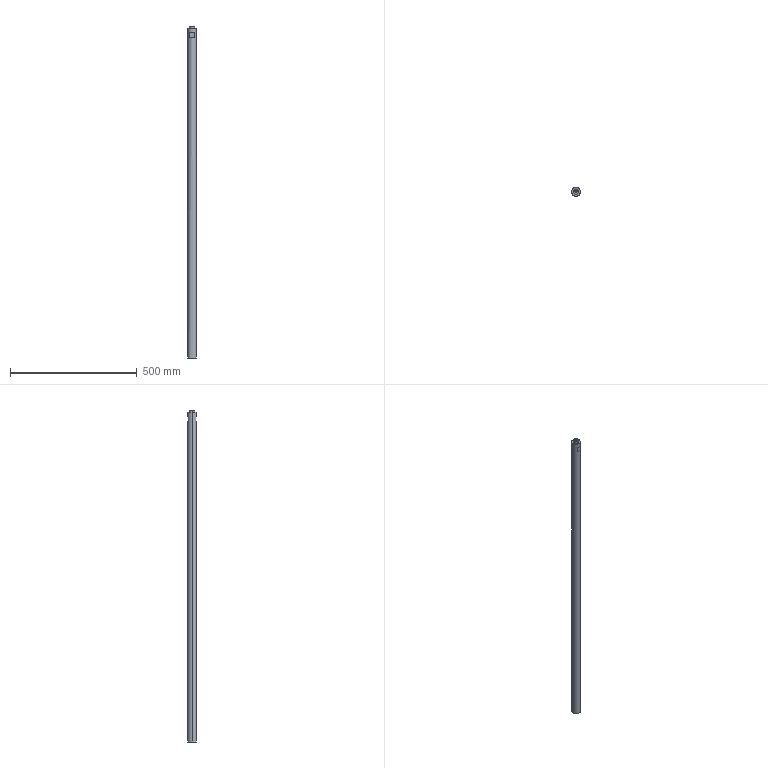Part | STEP file | 44-02-05 Press-fit Guide Shaft | 1 solid | 21 faces | box 35 x 35 x 1310 mm | volume 1250098 mm3 | plane 9 | cylinder 8 | cone 4 | commonest cylinder face diameters 8.5 x4 20 x2 35 x2
STEP:
#1=CARTESIAN_POINT('',(0.,0.,0.));
#2=DIRECTION('',(0.,0.,1.));
#3=DIRECTION('',(1.,0.,0.));
#4=AXIS2_PLACEMENT_3D('',#1,#2,#3);
#5=CARTESIAN_POINT('',(4.25,0.,627.5));
#6=VERTEX_POINT('',#5);
#7=CARTESIAN_POINT('',(4.25,0.,655.));
#8=VERTEX_POINT('',#7);
#9=CARTESIAN_POINT('',(4.25,0.,655.));
#10=DIRECTION('',(0.,0.,1.));
#11=VECTOR('',#10,1.);
#12=LINE('',#9,#11);
#13=CARTESIAN_POINT('',(0.,0.,655.));
#14=DIRECTION('',(0.,0.,1.));
#15=DIRECTION('',(1.,0.,0.));
#16=AXIS2_PLACEMENT_3D('',#13,#14,#15);
#17=CYLINDRICAL_SURFACE('',#16,4.25);
#18=CARTESIAN_POINT('',(6.283,0.));
#19=DIRECTION('',(0.,1.));
#20=VECTOR('',#19,1.);
#21=LINE('',#18,#20);
#22=(GEOMETRIC_REPRESENTATION_CONTEXT(2)PARAMETRIC_REPRESENTATION_CONTEXT()REPRESENTATION_CONTEXT('',''));
#23=DEFINITIONAL_REPRESENTATION('',(#21),#22);
#24=PCURVE('',#17,#23);
#25=CARTESIAN_POINT('',(0.,0.,655.));
#26=DIRECTION('',(0.,0.,1.));
#27=DIRECTION('',(1.,0.,0.));
#28=AXIS2_PLACEMENT_3D('',#25,#26,#27);
#29=CYLINDRICAL_SURFACE('',#28,4.25);
#30=CARTESIAN_POINT('',(0.,0.));
#31=DIRECTION('',(0.,1.));
#32=VECTOR('',#31,1.);
#33=LINE('',#30,#32);
#34=(GEOMETRIC_REPRESENTATION_CONTEXT(2)PARAMETRIC_REPRESENTATION_CONTEXT()REPRESENTATION_CONTEXT('',''));
#35=DEFINITIONAL_REPRESENTATION('',(#33),#34);
#36=PCURVE('',#29,#35);
#37=SURFACE_CURVE('',#12,(#24,#36),.PCURVE_S1.);
#38=EDGE_CURVE('',#6,#8,#37,.T.);
#39=ORIENTED_EDGE('',*,*,#38,.T.);
#40=CARTESIAN_POINT('',(-4.25,0.,655.));
#41=VERTEX_POINT('',#40);
#42=CARTESIAN_POINT('',(0.,0.,655.));
#43=DIRECTION('',(0.,0.,1.));
#44=DIRECTION('',(1.,0.,0.));
#45=AXIS2_PLACEMENT_3D('',#42,#43,#44);
#46=CIRCLE('',#45,4.25);
#47=CARTESIAN_POINT('',(0.,0.));
#48=DIRECTION('',(1.,0.));
#49=VECTOR('',#48,1.);
#50=LINE('',#47,#49);
#51=(GEOMETRIC_REPRESENTATION_CONTEXT(2)PARAMETRIC_REPRESENTATION_CONTEXT()REPRESENTATION_CONTEXT('',''));
#52=DEFINITIONAL_REPRESENTATION('',(#50),#51);
#53=PCURVE('',#17,#52);
#54=CARTESIAN_POINT('',(0.,0.,655.));
#55=DIRECTION('',(0.,0.,1.));
#56=DIRECTION('',(1.,0.,0.));
#57=AXIS2_PLACEMENT_3D('',#54,#55,#56);
#58=PLANE('',#57);
#59=CARTESIAN_POINT('',(0.,0.));
#60=DIRECTION('',(1.,0.));
#61=AXIS2_PLACEMENT_2D('',#59,#60);
#62=CIRCLE('',#61,4.25);
#63=(GEOMETRIC_REPRESENTATION_CONTEXT(2)PARAMETRIC_REPRESENTATION_CONTEXT()REPRESENTATION_CONTEXT('',''));
#64=DEFINITIONAL_REPRESENTATION('',(#62),#63);
#65=PCURVE('',#58,#64);
#66=SURFACE_CURVE('',#46,(#53,#65),.PCURVE_S1.);
#67=EDGE_CURVE('',#41,#8,#66,.T.);
#68=ORIENTED_EDGE('',*,*,#67,.F.);
#69=CARTESIAN_POINT('',(-4.25,0.,627.5));
#70=VERTEX_POINT('',#69);
#71=CARTESIAN_POINT('',(-4.25,0.,655.));
#72=DIRECTION('',(0.,0.,1.));
#73=VECTOR('',#72,1.);
#74=LINE('',#71,#73);
#75=CARTESIAN_POINT('',(3.142,0.));
#76=DIRECTION('',(0.,1.));
#77=VECTOR('',#76,1.);
#78=LINE('',#75,#77);
#79=(GEOMETRIC_REPRESENTATION_CONTEXT(2)PARAMETRIC_REPRESENTATION_CONTEXT()REPRESENTATION_CONTEXT('',''));
#80=DEFINITIONAL_REPRESENTATION('',(#78),#79);
#81=PCURVE('',#17,#80);
#82=CARTESIAN_POINT('',(3.142,0.));
#83=DIRECTION('',(0.,1.));
#84=VECTOR('',#83,1.);
#85=LINE('',#82,#84);
#86=(GEOMETRIC_REPRESENTATION_CONTEXT(2)PARAMETRIC_REPRESENTATION_CONTEXT()REPRESENTATION_CONTEXT('',''));
#87=DEFINITIONAL_REPRESENTATION('',(#85),#86);
#88=PCURVE('',#29,#87);
#89=SURFACE_CURVE('',#74,(#81,#88),.PCURVE_S1.);
#90=EDGE_CURVE('',#70,#41,#89,.T.);
#91=ORIENTED_EDGE('',*,*,#90,.F.);
#92=CARTESIAN_POINT('',(0.,0.,627.5));
#93=DIRECTION('',(0.,0.,1.));
#94=DIRECTION('',(1.,0.,0.));
#95=AXIS2_PLACEMENT_3D('',#92,#93,#94);
#96=CIRCLE('',#95,4.25);
#97=CARTESIAN_POINT('',(0.,-27.5));
#98=DIRECTION('',(1.,0.));
#99=VECTOR('',#98,1.);
#100=LINE('',#97,#99);
#101=(GEOMETRIC_REPRESENTATION_CONTEXT(2)PARAMETRIC_REPRESENTATION_CONTEXT()REPRESENTATION_CONTEXT('',''));
#102=DEFINITIONAL_REPRESENTATION('',(#100),#101);
#103=PCURVE('',#17,#102);
#104=CARTESIAN_POINT('',(0.,0.,627.5));
#105=DIRECTION('',(0.,0.,1.));
#106=DIRECTION('',(1.,0.,0.));
#107=AXIS2_PLACEMENT_3D('',#104,#105,#106);
#108=CONICAL_SURFACE('',#107,4.25,1.03);
#109=CARTESIAN_POINT('',(0.,0.));
#110=DIRECTION('',(1.,0.));
#111=VECTOR('',#110,1.);
#112=LINE('',#109,#111);
#113=(GEOMETRIC_REPRESENTATION_CONTEXT(2)PARAMETRIC_REPRESENTATION_CONTEXT()REPRESENTATION_CONTEXT('',''));
#114=DEFINITIONAL_REPRESENTATION('',(#112),#113);
#115=PCURVE('',#108,#114);
#116=SURFACE_CURVE('',#96,(#103,#115),.PCURVE_S1.);
#117=EDGE_CURVE('',#70,#6,#116,.T.);
#118=ORIENTED_EDGE('',*,*,#117,.T.);
#119=EDGE_LOOP('',(#39,#68,#91,#118));
#120=FACE_BOUND('',#119,.F.);
#121=ADVANCED_FACE('',(#120),#17,.F.);
#122=ORIENTED_EDGE('',*,*,#117,.F.);
#123=CARTESIAN_POINT('',(0.,0.,624.946));
#124=VERTEX_POINT('',#123);
#125=CARTESIAN_POINT('',(-4.25,0.,627.5));
#126=DIRECTION('',(-0.8572,0.,0.515));
#127=VECTOR('',#126,1.);
#128=LINE('',#125,#127);
#129=CARTESIAN_POINT('',(3.142,0.));
#130=DIRECTION('',(0.,1.));
#131=VECTOR('',#130,1.);
#132=LINE('',#129,#131);
#133=(GEOMETRIC_REPRESENTATION_CONTEXT(2)PARAMETRIC_REPRESENTATION_CONTEXT()REPRESENTATION_CONTEXT('',''));
#134=DEFINITIONAL_REPRESENTATION('',(#132),#133);
#135=PCURVE('',#108,#134);
#136=CARTESIAN_POINT('',(0.,0.,627.5));
#137=DIRECTION('',(0.,0.,1.));
#138=DIRECTION('',(1.,0.,0.));
#139=AXIS2_PLACEMENT_3D('',#136,#137,#138);
#140=CONICAL_SURFACE('',#139,4.25,1.03);
#141=CARTESIAN_POINT('',(3.142,0.));
#142=DIRECTION('',(0.,1.));
#143=VECTOR('',#142,1.);
#144=LINE('',#141,#143);
#145=(GEOMETRIC_REPRESENTATION_CONTEXT(2)PARAMETRIC_REPRESENTATION_CONTEXT()REPRESENTATION_CONTEXT('',''));
#146=DEFINITIONAL_REPRESENTATION('',(#144),#145);
#147=PCURVE('',#140,#146);
#148=SURFACE_CURVE('',#128,(#135,#147),.PCURVE_S1.);
#149=EDGE_CURVE('',#124,#70,#148,.T.);
#150=ORIENTED_EDGE('',*,*,#149,.F.);
#151=CARTESIAN_POINT('',(4.25,0.,627.5));
#152=DIRECTION('',(0.8572,0.,0.515));
#153=VECTOR('',#152,1.);
#154=LINE('',#151,#153);
#155=CARTESIAN_POINT('',(6.283,0.));
#156=DIRECTION('',(0.,1.));
#157=VECTOR('',#156,1.);
#158=LINE('',#155,#157);
#159=(GEOMETRIC_REPRESENTATION_CONTEXT(2)PARAMETRIC_REPRESENTATION_CONTEXT()REPRESENTATION_CONTEXT('',''));
#160=DEFINITIONAL_REPRESENTATION('',(#158),#159);
#161=PCURVE('',#108,#160);
#162=CARTESIAN_POINT('',(0.,0.));
#163=DIRECTION('',(0.,1.));
#164=VECTOR('',#163,1.);
#165=LINE('',#162,#164);
#166=(GEOMETRIC_REPRESENTATION_CONTEXT(2)PARAMETRIC_REPRESENTATION_CONTEXT()REPRESENTATION_CONTEXT('',''));
#167=DEFINITIONAL_REPRESENTATION('',(#165),#166);
#168=PCURVE('',#140,#167);
#169=SURFACE_CURVE('',#154,(#161,#168),.PCURVE_S1.);
#170=EDGE_CURVE('',#124,#6,#169,.T.);
#171=ORIENTED_EDGE('',*,*,#170,.T.);
#172=EDGE_LOOP('',(#122,#150,#171));
#173=FACE_BOUND('',#172,.F.);
#174=ADVANCED_FACE('',(#173),#108,.F.);
#175=CARTESIAN_POINT('',(10.,0.,646.));
#176=VERTEX_POINT('',#175);
#177=CARTESIAN_POINT('',(-10.,0.,646.));
#178=VERTEX_POINT('',#177);
#179=CARTESIAN_POINT('',(0.,0.,646.));
#180=DIRECTION('',(0.,0.,1.));
#181=DIRECTION('',(1.,0.,0.));
#182=AXIS2_PLACEMENT_3D('',#179,#180,#181);
#183=CIRCLE('',#182,10.);
#184=CARTESIAN_POINT('',(0.,0.,646.));
#185=DIRECTION('',(0.,0.,1.));
#186=DIRECTION('',(1.,0.,0.));
#187=AXIS2_PLACEMENT_3D('',#184,#185,#186);
#188=CYLINDRICAL_SURFACE('',#187,10.);
#189=CARTESIAN_POINT('',(0.,0.));
#190=DIRECTION('',(1.,0.));
#191=VECTOR('',#190,1.);
#192=LINE('',#189,#191);
#193=(GEOMETRIC_REPRESENTATION_CONTEXT(2)PARAMETRIC_REPRESENTATION_CONTEXT()REPRESENTATION_CONTEXT('',''));
#194=DEFINITIONAL_REPRESENTATION('',(#192),#193);
#195=PCURVE('',#188,#194);
#196=CARTESIAN_POINT('',(0.,0.,646.));
#197=DIRECTION('',(0.,0.,1.));
#198=DIRECTION('',(1.,0.,0.));
#199=AXIS2_PLACEMENT_3D('',#196,#197,#198);
#200=PLANE('',#199);
#201=CARTESIAN_POINT('',(0.,0.));
#202=DIRECTION('',(1.,0.));
#203=AXIS2_PLACEMENT_2D('',#201,#202);
#204=CIRCLE('',#203,10.);
#205=(GEOMETRIC_REPRESENTATION_CONTEXT(2)PARAMETRIC_REPRESENTATION_CONTEXT()REPRESENTATION_CONTEXT('',''));
#206=DEFINITIONAL_REPRESENTATION('',(#204),#205);
#207=PCURVE('',#200,#206);
#208=SURFACE_CURVE('',#183,(#195,#207),.PCURVE_S1.);
#209=EDGE_CURVE('',#176,#178,#208,.T.);
#210=ORIENTED_EDGE('',*,*,#209,.T.);
#211=CARTESIAN_POINT('',(-10.,0.,655.));
#212=VERTEX_POINT('',#211);
#213=CARTESIAN_POINT('',(-10.,0.,646.));
#214=DIRECTION('',(0.,0.,1.));
#215=VECTOR('',#214,1.);
#216=LINE('',#213,#215);
#217=CARTESIAN_POINT('',(3.142,0.));
#218=DIRECTION('',(0.,1.));
#219=VECTOR('',#218,1.);
#220=LINE('',#217,#219);
#221=(GEOMETRIC_REPRESENTATION_CONTEXT(2)PARAMETRIC_REPRESENTATION_CONTEXT()REPRESENTATION_CONTEXT('',''));
#222=DEFINITIONAL_REPRESENTATION('',(#220),#221);
#223=PCURVE('',#188,#222);
#224=CARTESIAN_POINT('',(0.,0.,646.));
#225=DIRECTION('',(0.,0.,1.));
#226=DIRECTION('',(1.,0.,0.));
#227=AXIS2_PLACEMENT_3D('',#224,#225,#226);
#228=CYLINDRICAL_SURFACE('',#227,10.);
#229=CARTESIAN_POINT('',(3.142,0.));
#230=DIRECTION('',(0.,1.));
#231=VECTOR('',#230,1.);
#232=LINE('',#229,#231);
#233=(GEOMETRIC_REPRESENTATION_CONTEXT(2)PARAMETRIC_REPRESENTATION_CONTEXT()REPRESENTATION_CONTEXT('',''));
#234=DEFINITIONAL_REPRESENTATION('',(#232),#233);
#235=PCURVE('',#228,#234);
#236=SURFACE_CURVE('',#216,(#223,#235),.PCURVE_S1.);
#237=EDGE_CURVE('',#178,#212,#236,.T.);
#238=ORIENTED_EDGE('',*,*,#237,.T.);
#239=CARTESIAN_POINT('',(10.,0.,655.));
#240=VERTEX_POINT('',#239);
#241=CARTESIAN_POINT('',(0.,0.,655.));
#242=DIRECTION('',(0.,0.,1.));
#243=DIRECTION('',(1.,0.,0.));
#244=AXIS2_PLACEMENT_3D('',#241,#242,#243);
#245=CIRCLE('',#244,10.);
#246=CARTESIAN_POINT('',(0.,9.));
#247=DIRECTION('',(1.,0.));
#248=VECTOR('',#247,1.);
#249=LINE('',#246,#248);
#250=(GEOMETRIC_REPRESENTATION_CONTEXT(2)PARAMETRIC_REPRESENTATION_CONTEXT()REPRESENTATION_CONTEXT('',''));
#251=DEFINITIONAL_REPRESENTATION('',(#249),#250);
#252=PCURVE('',#188,#251);
#253=CARTESIAN_POINT('',(0.,0.));
#254=DIRECTION('',(1.,0.));
#255=AXIS2_PLACEMENT_2D('',#253,#254);
#256=CIRCLE('',#255,10.);
#257=(GEOMETRIC_REPRESENTATION_CONTEXT(2)PARAMETRIC_REPRESENTATION_CONTEXT()REPRESENTATION_CONTEXT('',''));
#258=DEFINITIONAL_REPRESENTATION('',(#256),#257);
#259=PCURVE('',#58,#258);
#260=SURFACE_CURVE('',#245,(#252,#259),.PCURVE_S1.);
#261=EDGE_CURVE('',#240,#212,#260,.T.);
#262=ORIENTED_EDGE('',*,*,#261,.F.);
#263=CARTESIAN_POINT('',(10.,0.,646.));
#264=DIRECTION('',(0.,0.,1.));
#265=VECTOR('',#264,1.);
#266=LINE('',#263,#265);
#267=CARTESIAN_POINT('',(0.,0.));
#268=DIRECTION('',(0.,1.));
#269=VECTOR('',#268,1.);
#270=LINE('',#267,#269);
#271=(GEOMETRIC_REPRESENTATION_CONTEXT(2)PARAMETRIC_REPRESENTATION_CONTEXT()REPRESENTATION_CONTEXT('',''));
#272=DEFINITIONAL_REPRESENTATION('',(#270),#271);
#273=PCURVE('',#188,#272);
#274=CARTESIAN_POINT('',(6.283,0.));
#275=DIRECTION('',(0.,1.));
#276=VECTOR('',#275,1.);
#277=LINE('',#274,#276);
#278=(GEOMETRIC_REPRESENTATION_CONTEXT(2)PARAMETRIC_REPRESENTATION_CONTEXT()REPRESENTATION_CONTEXT('',''));
#279=DEFINITIONAL_REPRESENTATION('',(#277),#278);
#280=PCURVE('',#228,#279);
#281=SURFACE_CURVE('',#266,(#273,#280),.PCURVE_S1.);
#282=EDGE_CURVE('',#176,#240,#281,.T.);
#283=ORIENTED_EDGE('',*,*,#282,.F.);
#284=EDGE_LOOP('',(#210,#238,#262,#283));
#285=FACE_BOUND('',#284,.T.);
#286=ADVANCED_FACE('',(#285),#188,.T.);
#287=CARTESIAN_POINT('',(-4.25,0.,-627.5));
#288=VERTEX_POINT('',#287);
#289=CARTESIAN_POINT('',(-4.25,0.,-655.));
#290=VERTEX_POINT('',#289);
#291=CARTESIAN_POINT('',(-4.25,0.,-655.));
#292=DIRECTION('',(0.,0.,-1.));
#293=VECTOR('',#292,1.);
#294=LINE('',#291,#293);
#295=CARTESIAN_POINT('',(0.,0.,-655.));
#296=DIRECTION('',(0.,0.,-1.));
#297=DIRECTION('',(-1.,0.,0.));
#298=AXIS2_PLACEMENT_3D('',#295,#296,#297);
#299=CYLINDRICAL_SURFACE('',#298,4.25);
#300=CARTESIAN_POINT('',(6.283,0.));
#301=DIRECTION('',(0.,1.));
#302=VECTOR('',#301,1.);
#303=LINE('',#300,#302);
#304=(GEOMETRIC_REPRESENTATION_CONTEXT(2)PARAMETRIC_REPRESENTATION_CONTEXT()REPRESENTATION_CONTEXT('',''));
#305=DEFINITIONAL_REPRESENTATION('',(#303),#304);
#306=PCURVE('',#299,#305);
#307=CARTESIAN_POINT('',(0.,0.,-655.));
#308=DIRECTION('',(0.,0.,-1.));
#309=DIRECTION('',(-1.,0.,0.));
#310=AXIS2_PLACEMENT_3D('',#307,#308,#309);
#311=CYLINDRICAL_SURFACE('',#310,4.25);
#312=CARTESIAN_POINT('',(0.,0.));
#313=DIRECTION('',(0.,1.));
#314=VECTOR('',#313,1.);
#315=LINE('',#312,#314);
#316=(GEOMETRIC_REPRESENTATION_CONTEXT(2)PARAMETRIC_REPRESENTATION_CONTEXT()REPRESENTATION_CONTEXT('',''));
#317=DEFINITIONAL_REPRESENTATION('',(#315),#316);
#318=PCURVE('',#311,#317);
#319=SURFACE_CURVE('',#294,(#306,#318),.PCURVE_S1.);
#320=EDGE_CURVE('',#288,#290,#319,.T.);
#321=ORIENTED_EDGE('',*,*,#320,.T.);
#322=CARTESIAN_POINT('',(4.25,0.,-655.));
#323=VERTEX_POINT('',#322);
#324=CARTESIAN_POINT('',(0.,0.,-655.));
#325=DIRECTION('',(0.,0.,-1.));
#326=DIRECTION('',(-1.,0.,0.));
#327=AXIS2_PLACEMENT_3D('',#324,#325,#326);
#328=CIRCLE('',#327,4.25);
#329=CARTESIAN_POINT('',(0.,0.));
#330=DIRECTION('',(1.,0.));
#331=VECTOR('',#330,1.);
#332=LINE('',#329,#331);
#333=(GEOMETRIC_REPRESENTATION_CONTEXT(2)PARAMETRIC_REPRESENTATION_CONTEXT()REPRESENTATION_CONTEXT('',''));
#334=DEFINITIONAL_REPRESENTATION('',(#332),#333);
#335=PCURVE('',#299,#334);
#336=CARTESIAN_POINT('',(0.,0.,-655.));
#337=DIRECTION('',(0.,0.,1.));
#338=DIRECTION('',(1.,0.,0.));
#339=AXIS2_PLACEMENT_3D('',#336,#337,#338);
#340=PLANE('',#339);
#341=CARTESIAN_POINT('',(-4.25,0.));
#342=CARTESIAN_POINT('',(-4.25,7.361));
#343=CARTESIAN_POINT('',(2.125,3.681));
#344=CARTESIAN_POINT('',(8.5,0.));
#345=CARTESIAN_POINT('',(2.125,-3.681));
#346=CARTESIAN_POINT('',(-4.25,-7.361));
#347=CARTESIAN_POINT('',(-4.25,0.));
#348=(BOUNDED_CURVE()B_SPLINE_CURVE(2,(#341,#342,#343,#344,#345,#346,#347),.UNSPECIFIED.,.T.,.F.)B_SPLINE_CURVE_WITH_KNOTS((1,2,2,2,2,1),(-2.094,0.,2.094,4.189,6.283,8.378),.UNSPECIFIED.)CURVE()GEOMETRIC_REPRESENTATION_ITEM()RATIONAL_B_SPLINE_CURVE((1.,0.5,1.,0.5,1.,0.5,1.))REPRESENTATION_ITEM(''));
#349=(GEOMETRIC_REPRESENTATION_CONTEXT(2)PARAMETRIC_REPRESENTATION_CONTEXT()REPRESENTATION_CONTEXT('',''));
#350=DEFINITIONAL_REPRESENTATION('',(#348),#349);
#351=PCURVE('',#340,#350);
#352=SURFACE_CURVE('',#328,(#335,#351),.PCURVE_S1.);
#353=EDGE_CURVE('',#323,#290,#352,.T.);
#354=ORIENTED_EDGE('',*,*,#353,.F.);
#355=CARTESIAN_POINT('',(4.25,0.,-627.5));
#356=VERTEX_POINT('',#355);
#357=CARTESIAN_POINT('',(4.25,0.,-655.));
#358=DIRECTION('',(0.,0.,-1.));
#359=VECTOR('',#358,1.);
#360=LINE('',#357,#359);
#361=CARTESIAN_POINT('',(3.142,0.));
#362=DIRECTION('',(0.,1.));
#363=VECTOR('',#362,1.);
#364=LINE('',#361,#363);
#365=(GEOMETRIC_REPRESENTATION_CONTEXT(2)PARAMETRIC_REPRESENTATION_CONTEXT()REPRESENTATION_CONTEXT('',''));
#366=DEFINITIONAL_REPRESENTATION('',(#364),#365);
#367=PCURVE('',#299,#366);
#368=CARTESIAN_POINT('',(3.142,0.));
#369=DIRECTION('',(0.,1.));
#370=VECTOR('',#369,1.);
#371=LINE('',#368,#370);
#372=(GEOMETRIC_REPRESENTATION_CONTEXT(2)PARAMETRIC_REPRESENTATION_CONTEXT()REPRESENTATION_CONTEXT('',''));
#373=DEFINITIONAL_REPRESENTATION('',(#371),#372);
#374=PCURVE('',#311,#373);
#375=SURFACE_CURVE('',#360,(#367,#374),.PCURVE_S1.);
#376=EDGE_CURVE('',#356,#323,#375,.T.);
#377=ORIENTED_EDGE('',*,*,#376,.F.);
#378=CARTESIAN_POINT('',(0.,0.,-627.5));
#379=DIRECTION('',(0.,0.,-1.));
#380=DIRECTION('',(-1.,0.,0.));
#381=AXIS2_PLACEMENT_3D('',#378,#379,#380);
#382=CIRCLE('',#381,4.25);
#383=CARTESIAN_POINT('',(0.,-27.5));
#384=DIRECTION('',(1.,0.));
#385=VECTOR('',#384,1.);
#386=LINE('',#383,#385);
#387=(GEOMETRIC_REPRESENTATION_CONTEXT(2)PARAMETRIC_REPRESENTATION_CONTEXT()REPRESENTATION_CONTEXT('',''));
#388=DEFINITIONAL_REPRESENTATION('',(#386),#387);
#389=PCURVE('',#299,#388);
#390=CARTESIAN_POINT('',(0.,0.,-627.5));
#391=DIRECTION('',(0.,0.,-1.));
#392=DIRECTION('',(-1.,0.,0.));
#393=AXIS2_PLACEMENT_3D('',#390,#391,#392);
#394=CONICAL_SURFACE('',#393,4.25,1.03);
#395=CARTESIAN_POINT('',(0.,0.));
#396=DIRECTION('',(1.,0.));
#397=VECTOR('',#396,1.);
#398=LINE('',#395,#397);
#399=(GEOMETRIC_REPRESENTATION_CONTEXT(2)PARAMETRIC_REPRESENTATION_CONTEXT()REPRESENTATION_CONTEXT('',''));
#400=DEFINITIONAL_REPRESENTATION('',(#398),#399);
#401=PCURVE('',#394,#400);
#402=SURFACE_CURVE('',#382,(#389,#401),.PCURVE_S1.);
#403=EDGE_CURVE('',#356,#288,#402,.T.);
#404=ORIENTED_EDGE('',*,*,#403,.T.);
#405=EDGE_LOOP('',(#321,#354,#377,#404));
#406=FACE_BOUND('',#405,.F.);
#407=ADVANCED_FACE('',(#406),#299,.F.);
#408=ORIENTED_EDGE('',*,*,#403,.F.);
#409=CARTESIAN_POINT('',(0.,0.,-624.946));
#410=VERTEX_POINT('',#409);
#411=CARTESIAN_POINT('',(4.25,0.,-627.5));
#412=DIRECTION('',(0.8572,0.,-0.515));
#413=VECTOR('',#412,1.);
#414=LINE('',#411,#413);
#415=CARTESIAN_POINT('',(3.142,0.));
#416=DIRECTION('',(0.,1.));
#417=VECTOR('',#416,1.);
#418=LINE('',#415,#417);
#419=(GEOMETRIC_REPRESENTATION_CONTEXT(2)PARAMETRIC_REPRESENTATION_CONTEXT()REPRESENTATION_CONTEXT('',''));
#420=DEFINITIONAL_REPRESENTATION('',(#418),#419);
#421=PCURVE('',#394,#420);
#422=CARTESIAN_POINT('',(0.,0.,-627.5));
#423=DIRECTION('',(0.,0.,-1.));
#424=DIRECTION('',(-1.,0.,0.));
#425=AXIS2_PLACEMENT_3D('',#422,#423,#424);
#426=CONICAL_SURFACE('',#425,4.25,1.03);
#427=CARTESIAN_POINT('',(3.142,0.));
#428=DIRECTION('',(0.,1.));
#429=VECTOR('',#428,1.);
#430=LINE('',#427,#429);
#431=(GEOMETRIC_REPRESENTATION_CONTEXT(2)PARAMETRIC_REPRESENTATION_CONTEXT()REPRESENTATION_CONTEXT('',''));
#432=DEFINITIONAL_REPRESENTATION('',(#430),#431);
#433=PCURVE('',#426,#432);
#434=SURFACE_CURVE('',#414,(#421,#433),.PCURVE_S1.);
#435=EDGE_CURVE('',#410,#356,#434,.T.);
#436=ORIENTED_EDGE('',*,*,#435,.F.);
#437=CARTESIAN_POINT('',(-4.25,0.,-627.5));
#438=DIRECTION('',(-0.8572,0.,-0.515));
#439=VECTOR('',#438,1.);
#440=LINE('',#437,#439);
#441=CARTESIAN_POINT('',(6.283,0.));
#442=DIRECTION('',(0.,1.));
#443=VECTOR('',#442,1.);
#444=LINE('',#441,#443);
#445=(GEOMETRIC_REPRESENTATION_CONTEXT(2)PARAMETRIC_REPRESENTATION_CONTEXT()REPRESENTATION_CONTEXT('',''));
#446=DEFINITIONAL_REPRESENTATION('',(#444),#445);
#447=PCURVE('',#394,#446);
#448=CARTESIAN_POINT('',(0.,0.));
#449=DIRECTION('',(0.,1.));
#450=VECTOR('',#449,1.);
#451=LINE('',#448,#450);
#452=(GEOMETRIC_REPRESENTATION_CONTEXT(2)PARAMETRIC_REPRESENTATION_CONTEXT()REPRESENTATION_CONTEXT('',''));
#453=DEFINITIONAL_REPRESENTATION('',(#451),#452);
#454=PCURVE('',#426,#453);
#455=SURFACE_CURVE('',#440,(#447,#454),.PCURVE_S1.);
#456=EDGE_CURVE('',#410,#288,#455,.T.);
#457=ORIENTED_EDGE('',*,*,#456,.T.);
#458=EDGE_LOOP('',(#408,#436,#457));
#459=FACE_BOUND('',#458,.F.);
#460=ADVANCED_FACE('',(#459),#394,.F.);
#461=CARTESIAN_POINT('',(9.014,15.,630.));
#462=VERTEX_POINT('',#461);
#463=CARTESIAN_POINT('',(9.014,15.,610.));
#464=VERTEX_POINT('',#463);
#465=CARTESIAN_POINT('',(9.014,15.,655.));
#466=DIRECTION('',(0.,0.,-1.));
#467=VECTOR('',#466,1.);
#468=LINE('',#465,#467);
#469=CARTESIAN_POINT('',(0.,0.,655.));
#470=DIRECTION('',(0.,0.,-1.));
#471=DIRECTION('',(-1.,0.,0.));
#472=AXIS2_PLACEMENT_3D('',#469,#470,#471);
#473=CYLINDRICAL_SURFACE('',#472,17.5);
#474=CARTESIAN_POINT('',(2.112,0.));
#475=DIRECTION('',(0.,1.));
#476=VECTOR('',#475,1.);
#477=LINE('',#474,#476);
#478=(GEOMETRIC_REPRESENTATION_CONTEXT(2)PARAMETRIC_REPRESENTATION_CONTEXT()REPRESENTATION_CONTEXT('',''));
#479=DEFINITIONAL_REPRESENTATION('',(#477),#478);
#480=PCURVE('',#473,#479);
#481=CARTESIAN_POINT('',(38.348,15.,610.));
#482=DIRECTION('',(0.,1.,0.));
#483=DIRECTION('',(0.,0.,1.));
#484=AXIS2_PLACEMENT_3D('',#481,#482,#483);
#485=PLANE('',#484);
#486=CARTESIAN_POINT('',(45.,-29.334));
#487=DIRECTION('',(-1.,0.));
#488=VECTOR('',#487,1.);
#489=LINE('',#486,#488);
#490=(GEOMETRIC_REPRESENTATION_CONTEXT(2)PARAMETRIC_REPRESENTATION_CONTEXT()REPRESENTATION_CONTEXT('',''));
#491=DEFINITIONAL_REPRESENTATION('',(#489),#490);
#492=PCURVE('',#485,#491);
#493=SURFACE_CURVE('',#468,(#480,#492),.PCURVE_S1.);
#494=EDGE_CURVE('',#462,#464,#493,.T.);
#495=ORIENTED_EDGE('',*,*,#494,.F.);
#496=CARTESIAN_POINT('',(-9.014,15.,630.));
#497=VERTEX_POINT('',#496);
#498=CARTESIAN_POINT('',(0.,0.,630.));
#499=DIRECTION('',(0.,0.,1.));
#500=DIRECTION('',(1.,0.,0.));
#501=AXIS2_PLACEMENT_3D('',#498,#499,#500);
#502=CIRCLE('',#501,17.5);
#503=CARTESIAN_POINT('',(3.142,25.));
#504=DIRECTION('',(-1.,0.));
#505=VECTOR('',#504,1.);
#506=LINE('',#503,#505);
#507=(GEOMETRIC_REPRESENTATION_CONTEXT(2)PARAMETRIC_REPRESENTATION_CONTEXT()REPRESENTATION_CONTEXT('',''));
#508=DEFINITIONAL_REPRESENTATION('',(#506),#507);
#509=PCURVE('',#473,#508);
#510=CARTESIAN_POINT('',(38.348,15.,630.));
#511=DIRECTION('',(0.,0.,1.));
#512=DIRECTION('',(1.,0.,0.));
#513=AXIS2_PLACEMENT_3D('',#510,#511,#512);
#514=PLANE('',#513);
#515=CARTESIAN_POINT('',(-38.348,-15.));
#516=DIRECTION('',(1.,0.));
#517=AXIS2_PLACEMENT_2D('',#515,#516);
#518=CIRCLE('',#517,17.5);
#519=(GEOMETRIC_REPRESENTATION_CONTEXT(2)PARAMETRIC_REPRESENTATION_CONTEXT()REPRESENTATION_CONTEXT('',''));
#520=DEFINITIONAL_REPRESENTATION('',(#518),#519);
#521=PCURVE('',#514,#520);
#522=SURFACE_CURVE('',#502,(#509,#521),.PCURVE_S1.);
#523=EDGE_CURVE('',#462,#497,#522,.T.);
#524=ORIENTED_EDGE('',*,*,#523,.T.);
#525=CARTESIAN_POINT('',(-9.014,15.,610.));
#526=VERTEX_POINT('',#525);
#527=CARTESIAN_POINT('',(-9.014,15.,655.));
#528=DIRECTION('',(0.,0.,1.));
#529=VECTOR('',#528,1.);
#530=LINE('',#527,#529);
#531=CARTESIAN_POINT('',(1.03,0.));
#532=DIRECTION('',(0.,-1.));
#533=VECTOR('',#532,1.);
#534=LINE('',#531,#533);
#535=(GEOMETRIC_REPRESENTATION_CONTEXT(2)PARAMETRIC_REPRESENTATION_CONTEXT()REPRESENTATION_CONTEXT('',''));
#536=DEFINITIONAL_REPRESENTATION('',(#534),#535);
#537=PCURVE('',#473,#536);
#538=CARTESIAN_POINT('',(45.,-47.362));
#539=DIRECTION('',(1.,0.));
#540=VECTOR('',#539,1.);
#541=LINE('',#538,#540);
#542=(GEOMETRIC_REPRESENTATION_CONTEXT(2)PARAMETRIC_REPRESENTATION_CONTEXT()REPRESENTATION_CONTEXT('',''));
#543=DEFINITIONAL_REPRESENTATION('',(#541),#542);
#544=PCURVE('',#485,#543);
#545=SURFACE_CURVE('',#530,(#537,#544),.PCURVE_S1.);
#546=EDGE_CURVE('',#526,#497,#545,.T.);
#547=ORIENTED_EDGE('',*,*,#546,.F.);
#548=CARTESIAN_POINT('',(0.,0.,610.));
#549=DIRECTION('',(0.,0.,-1.));
#550=DIRECTION('',(-1.,0.,0.));
#551=AXIS2_PLACEMENT_3D('',#548,#549,#550);
#552=CIRCLE('',#551,17.5);
#553=CARTESIAN_POINT('',(0.,45.));
#554=DIRECTION('',(1.,0.));
#555=VECTOR('',#554,1.);
#556=LINE('',#553,#555);
#557=(GEOMETRIC_REPRESENTATION_CONTEXT(2)PARAMETRIC_REPRESENTATION_CONTEXT()REPRESENTATION_CONTEXT('',''));
#558=DEFINITIONAL_REPRESENTATION('',(#556),#557);
#559=PCURVE('',#473,#558);
#560=CARTESIAN_POINT('',(38.348,15.,610.));
#561=DIRECTION('',(0.,0.,-1.));
#562=DIRECTION('',(-1.,0.,0.));
#563=AXIS2_PLACEMENT_3D('',#560,#561,#562);
#564=PLANE('',#563);
#565=CARTESIAN_POINT('',(38.348,-15.));
#566=DIRECTION('',(1.,0.));
#567=AXIS2_PLACEMENT_2D('',#565,#566);
#568=CIRCLE('',#567,17.5);
#569=(GEOMETRIC_REPRESENTATION_CONTEXT(2)PARAMETRIC_REPRESENTATION_CONTEXT()REPRESENTATION_CONTEXT('',''));
#570=DEFINITIONAL_REPRESENTATION('',(#568),#569);
#571=PCURVE('',#564,#570);
#572=SURFACE_CURVE('',#552,(#559,#571),.PCURVE_S1.);
#573=EDGE_CURVE('',#526,#464,#572,.T.);
#574=ORIENTED_EDGE('',*,*,#573,.T.);
#575=EDGE_LOOP('',(#495,#524,#547,#574));
#576=FACE_BOUND('',#575,.T.);
#577=CARTESIAN_POINT('',(17.5,0.,646.));
#578=VERTEX_POINT('',#577);
#579=CARTESIAN_POINT('',(-17.5,0.,646.));
#580=VERTEX_POINT('',#579);
#581=CARTESIAN_POINT('',(0.,0.,646.));
#582=DIRECTION('',(0.,0.,1.));
#583=DIRECTION('',(1.,0.,0.));
#584=AXIS2_PLACEMENT_3D('',#581,#582,#583);
#585=CIRCLE('',#584,17.5);
#586=CARTESIAN_POINT('',(3.142,9.));
#587=DIRECTION('',(-1.,0.));
#588=VECTOR('',#587,1.);
#589=LINE('',#586,#588);
#590=(GEOMETRIC_REPRESENTATION_CONTEXT(2)PARAMETRIC_REPRESENTATION_CONTEXT()REPRESENTATION_CONTEXT('',''));
#591=DEFINITIONAL_REPRESENTATION('',(#589),#590);
#592=PCURVE('',#473,#591);
#593=CARTESIAN_POINT('',(0.,0.));
#594=DIRECTION('',(1.,0.));
#595=AXIS2_PLACEMENT_2D('',#593,#594);
#596=CIRCLE('',#595,17.5);
#597=(GEOMETRIC_REPRESENTATION_CONTEXT(2)PARAMETRIC_REPRESENTATION_CONTEXT()REPRESENTATION_CONTEXT('',''));
#598=DEFINITIONAL_REPRESENTATION('',(#596),#597);
#599=PCURVE('',#200,#598);
#600=SURFACE_CURVE('',#585,(#592,#599),.PCURVE_S1.);
#601=EDGE_CURVE('',#578,#580,#600,.T.);
#602=ORIENTED_EDGE('',*,*,#601,.F.);
#603=CARTESIAN_POINT('',(17.5,0.,-655.));
#604=VERTEX_POINT('',#603);
#605=CARTESIAN_POINT('',(17.5,0.,655.));
#606=DIRECTION('',(0.,0.,-1.));
#607=VECTOR('',#606,1.);
#608=LINE('',#605,#607);
#609=CARTESIAN_POINT('',(3.142,0.));
#610=DIRECTION('',(0.,1.));
#611=VECTOR('',#610,1.);
#612=LINE('',#609,#611);
#613=(GEOMETRIC_REPRESENTATION_CONTEXT(2)PARAMETRIC_REPRESENTATION_CONTEXT()REPRESENTATION_CONTEXT('',''));
#614=DEFINITIONAL_REPRESENTATION('',(#612),#613);
#615=PCURVE('',#473,#614);
#616=CARTESIAN_POINT('',(0.,0.,655.));
#617=DIRECTION('',(0.,0.,-1.));
#618=DIRECTION('',(-1.,0.,0.));
#619=AXIS2_PLACEMENT_3D('',#616,#617,#618);
#620=CYLINDRICAL_SURFACE('',#619,17.5);
#621=CARTESIAN_POINT('',(3.142,0.));
#622=DIRECTION('',(0.,1.));
#623=VECTOR('',#622,1.);
#624=LINE('',#621,#623);
#625=(GEOMETRIC_REPRESENTATION_CONTEXT(2)PARAMETRIC_REPRESENTATION_CONTEXT()REPRESENTATION_CONTEXT('',''));
#626=DEFINITIONAL_REPRESENTATION('',(#624),#625);
#627=PCURVE('',#620,#626);
#628=SURFACE_CURVE('',#608,(#615,#627),.PCURVE_S1.);
#629=EDGE_CURVE('',#578,#604,#628,.T.);
#630=ORIENTED_EDGE('',*,*,#629,.T.);
#631=CARTESIAN_POINT('',(-17.5,0.,-655.));
#632=VERTEX_POINT('',#631);
#633=CARTESIAN_POINT('',(0.,0.,-655.));
#634=DIRECTION('',(0.,0.,1.));
#635=DIRECTION('',(1.,0.,0.));
#636=AXIS2_PLACEMENT_3D('',#633,#634,#635);
#637=CIRCLE('',#636,17.5);
#638=CARTESIAN_POINT('',(3.142,1310.));
#639=DIRECTION('',(-1.,0.));
#640=VECTOR('',#639,1.);
#641=LINE('',#638,#640);
#642=(GEOMETRIC_REPRESENTATION_CONTEXT(2)PARAMETRIC_REPRESENTATION_CONTEXT()REPRESENTATION_CONTEXT('',''));
#643=DEFINITIONAL_REPRESENTATION('',(#641),#642);
#644=PCURVE('',#473,#643);
#645=CARTESIAN_POINT('',(0.,0.));
#646=DIRECTION('',(1.,0.));
#647=AXIS2_PLACEMENT_2D('',#645,#646);
#648=CIRCLE('',#647,17.5);
#649=(GEOMETRIC_REPRESENTATION_CONTEXT(2)PARAMETRIC_REPRESENTATION_CONTEXT()REPRESENTATION_CONTEXT('',''));
#650=DEFINITIONAL_REPRESENTATION('',(#648),#649);
#651=PCURVE('',#340,#650);
#652=SURFACE_CURVE('',#637,(#644,#651),.PCURVE_S1.);
#653=EDGE_CURVE('',#604,#632,#652,.T.);
#654=ORIENTED_EDGE('',*,*,#653,.T.);
#655=CARTESIAN_POINT('',(-17.5,0.,655.));
#656=DIRECTION('',(0.,0.,-1.));
#657=VECTOR('',#656,1.);
#658=LINE('',#655,#657);
#659=CARTESIAN_POINT('',(0.,0.));
#660=DIRECTION('',(0.,1.));
#661=VECTOR('',#660,1.);
#662=LINE('',#659,#661);
#663=(GEOMETRIC_REPRESENTATION_CONTEXT(2)PARAMETRIC_REPRESENTATION_CONTEXT()REPRESENTATION_CONTEXT('',''));
#664=DEFINITIONAL_REPRESENTATION('',(#662),#663);
#665=PCURVE('',#473,#664);
#666=CARTESIAN_POINT('',(6.283,0.));
#667=DIRECTION('',(0.,1.));
#668=VECTOR('',#667,1.);
#669=LINE('',#666,#668);
#670=(GEOMETRIC_REPRESENTATION_CONTEXT(2)PARAMETRIC_REPRESENTATION_CONTEXT()REPRESENTATION_CONTEXT('',''));
#671=DEFINITIONAL_REPRESENTATION('',(#669),#670);
#672=PCURVE('',#620,#671);
#673=SURFACE_CURVE('',#658,(#665,#672),.PCURVE_S1.);
#674=EDGE_CURVE('',#580,#632,#673,.T.);
#675=ORIENTED_EDGE('',*,*,#674,.F.);
#676=EDGE_LOOP('',(#602,#630,#654,#675));
#677=FACE_BOUND('',#676,.T.);
#678=ADVANCED_FACE('',(#576,#677),#473,.T.);
#679=ORIENTED_EDGE('',*,*,#629,.F.);
#680=CARTESIAN_POINT('',(0.,0.,646.));
#681=DIRECTION('',(0.,0.,1.));
#682=DIRECTION('',(1.,0.,0.));
#683=AXIS2_PLACEMENT_3D('',#680,#681,#682);
#684=CIRCLE('',#683,17.5);
#685=CARTESIAN_POINT('',(9.425,9.));
#686=DIRECTION('',(-1.,0.));
#687=VECTOR('',#686,1.);
#688=LINE('',#685,#687);
#689=(GEOMETRIC_REPRESENTATION_CONTEXT(2)PARAMETRIC_REPRESENTATION_CONTEXT()REPRESENTATION_CONTEXT('',''));
#690=DEFINITIONAL_REPRESENTATION('',(#688),#689);
#691=PCURVE('',#620,#690);
#692=CARTESIAN_POINT('',(0.,0.));
#693=DIRECTION('',(1.,0.));
#694=AXIS2_PLACEMENT_2D('',#692,#693);
#695=CIRCLE('',#694,17.5);
#696=(GEOMETRIC_REPRESENTATION_CONTEXT(2)PARAMETRIC_REPRESENTATION_CONTEXT()REPRESENTATION_CONTEXT('',''));
#697=DEFINITIONAL_REPRESENTATION('',(#695),#696);
#698=PCURVE('',#200,#697);
#699=SURFACE_CURVE('',#684,(#691,#698),.PCURVE_S1.);
#700=EDGE_CURVE('',#580,#578,#699,.T.);
#701=ORIENTED_EDGE('',*,*,#700,.F.);
#702=ORIENTED_EDGE('',*,*,#674,.T.);
#703=CARTESIAN_POINT('',(0.,0.,-655.));
#704=DIRECTION('',(0.,0.,1.));
#705=DIRECTION('',(1.,0.,0.));
#706=AXIS2_PLACEMENT_3D('',#703,#704,#705);
#707=CIRCLE('',#706,17.5);
#708=CARTESIAN_POINT('',(9.425,1310.));
#709=DIRECTION('',(-1.,0.));
#710=VECTOR('',#709,1.);
#711=LINE('',#708,#710);
#712=(GEOMETRIC_REPRESENTATION_CONTEXT(2)PARAMETRIC_REPRESENTATION_CONTEXT()REPRESENTATION_CONTEXT('',''));
#713=DEFINITIONAL_REPRESENTATION('',(#711),#712);
#714=PCURVE('',#620,#713);
#715=CARTESIAN_POINT('',(0.,0.));
#716=DIRECTION('',(1.,0.));
#717=AXIS2_PLACEMENT_2D('',#715,#716);
#718=CIRCLE('',#717,17.5);
#719=(GEOMETRIC_REPRESENTATION_CONTEXT(2)PARAMETRIC_REPRESENTATION_CONTEXT()REPRESENTATION_CONTEXT('',''));
#720=DEFINITIONAL_REPRESENTATION('',(#718),#719);
#721=PCURVE('',#340,#720);
#722=SURFACE_CURVE('',#707,(#714,#721),.PCURVE_S1.);
#723=EDGE_CURVE('',#632,#604,#722,.T.);
#724=ORIENTED_EDGE('',*,*,#723,.T.);
#725=EDGE_LOOP('',(#679,#701,#702,#724));
#726=FACE_BOUND('',#725,.T.);
#727=CARTESIAN_POINT('',(-9.014,-15.,610.));
#728=VERTEX_POINT('',#727);
#729=CARTESIAN_POINT('',(9.014,-15.,610.));
#730=VERTEX_POINT('',#729);
#731=CARTESIAN_POINT('',(0.,0.,610.));
#732=DIRECTION('',(0.,0.,1.));
#733=DIRECTION('',(1.,0.,0.));
#734=AXIS2_PLACEMENT_3D('',#731,#732,#733);
#735=CIRCLE('',#734,17.5);
#736=CARTESIAN_POINT('',(9.425,45.));
#737=DIRECTION('',(-1.,0.));
#738=VECTOR('',#737,1.);
#739=LINE('',#736,#738);
#740=(GEOMETRIC_REPRESENTATION_CONTEXT(2)PARAMETRIC_REPRESENTATION_CONTEXT()REPRESENTATION_CONTEXT('',''));
#741=DEFINITIONAL_REPRESENTATION('',(#739),#740);
#742=PCURVE('',#620,#741);
#743=CARTESIAN_POINT('',(38.348,-15.,610.));
#744=DIRECTION('',(0.,0.,1.));
#745=DIRECTION('',(1.,0.,0.));
#746=AXIS2_PLACEMENT_3D('',#743,#744,#745);
#747=PLANE('',#746);
#748=CARTESIAN_POINT('',(-38.348,15.));
#749=DIRECTION('',(1.,0.));
#750=AXIS2_PLACEMENT_2D('',#748,#749);
#751=CIRCLE('',#750,17.5);
#752=(GEOMETRIC_REPRESENTATION_CONTEXT(2)PARAMETRIC_REPRESENTATION_CONTEXT()REPRESENTATION_CONTEXT('',''));
#753=DEFINITIONAL_REPRESENTATION('',(#751),#752);
#754=PCURVE('',#747,#753);
#755=SURFACE_CURVE('',#735,(#742,#754),.PCURVE_S1.);
#756=EDGE_CURVE('',#728,#730,#755,.T.);
#757=ORIENTED_EDGE('',*,*,#756,.F.);
#758=CARTESIAN_POINT('',(-9.014,-15.,630.));
#759=VERTEX_POINT('',#758);
#760=CARTESIAN_POINT('',(-9.014,-15.,655.));
#761=DIRECTION('',(0.,0.,-1.));
#762=VECTOR('',#761,1.);
#763=LINE('',#760,#762);
#764=CARTESIAN_POINT('',(5.253,0.));
#765=DIRECTION('',(0.,1.));
#766=VECTOR('',#765,1.);
#767=LINE('',#764,#766);
#768=(GEOMETRIC_REPRESENTATION_CONTEXT(2)PARAMETRIC_REPRESENTATION_CONTEXT()REPRESENTATION_CONTEXT('',''));
#769=DEFINITIONAL_REPRESENTATION('',(#767),#768);
#770=PCURVE('',#620,#769);
#771=CARTESIAN_POINT('',(38.348,-15.,610.));
#772=DIRECTION('',(0.,-1.,0.));
#773=DIRECTION('',(0.,0.,1.));
#774=AXIS2_PLACEMENT_3D('',#771,#772,#773);
#775=PLANE('',#774);
#776=CARTESIAN_POINT('',(45.,47.362));
#777=DIRECTION('',(-1.,0.));
#778=VECTOR('',#777,1.);
#779=LINE('',#776,#778);
#780=(GEOMETRIC_REPRESENTATION_CONTEXT(2)PARAMETRIC_REPRESENTATION_CONTEXT()REPRESENTATION_CONTEXT('',''));
#781=DEFINITIONAL_REPRESENTATION('',(#779),#780);
#782=PCURVE('',#775,#781);
#783=SURFACE_CURVE('',#763,(#770,#782),.PCURVE_S1.);
#784=EDGE_CURVE('',#759,#728,#783,.T.);
#785=ORIENTED_EDGE('',*,*,#784,.F.);
#786=CARTESIAN_POINT('',(9.014,-15.,630.));
#787=VERTEX_POINT('',#786);
#788=CARTESIAN_POINT('',(0.,0.,630.));
#789=DIRECTION('',(0.,0.,-1.));
#790=DIRECTION('',(-1.,0.,0.));
#791=AXIS2_PLACEMENT_3D('',#788,#789,#790);
#792=CIRCLE('',#791,17.5);
#793=CARTESIAN_POINT('',(0.,25.));
#794=DIRECTION('',(1.,0.));
#795=VECTOR('',#794,1.);
#796=LINE('',#793,#795);
#797=(GEOMETRIC_REPRESENTATION_CONTEXT(2)PARAMETRIC_REPRESENTATION_CONTEXT()REPRESENTATION_CONTEXT('',''));
#798=DEFINITIONAL_REPRESENTATION('',(#796),#797);
#799=PCURVE('',#620,#798);
#800=CARTESIAN_POINT('',(38.348,-15.,630.));
#801=DIRECTION('',(0.,0.,-1.));
#802=DIRECTION('',(-1.,0.,0.));
#803=AXIS2_PLACEMENT_3D('',#800,#801,#802);
#804=PLANE('',#803);
#805=CARTESIAN_POINT('',(38.348,15.));
#806=DIRECTION('',(1.,0.));
#807=AXIS2_PLACEMENT_2D('',#805,#806);
#808=CIRCLE('',#807,17.5);
#809=(GEOMETRIC_REPRESENTATION_CONTEXT(2)PARAMETRIC_REPRESENTATION_CONTEXT()REPRESENTATION_CONTEXT('',''));
#810=DEFINITIONAL_REPRESENTATION('',(#808),#809);
#811=PCURVE('',#804,#810);
#812=SURFACE_CURVE('',#792,(#799,#811),.PCURVE_S1.);
#813=EDGE_CURVE('',#787,#759,#812,.T.);
#814=ORIENTED_EDGE('',*,*,#813,.F.);
#815=CARTESIAN_POINT('',(9.014,-15.,655.));
#816=DIRECTION('',(0.,0.,1.));
#817=VECTOR('',#816,1.);
#818=LINE('',#815,#817);
#819=CARTESIAN_POINT('',(4.171,0.));
#820=DIRECTION('',(0.,-1.));
#821=VECTOR('',#820,1.);
#822=LINE('',#819,#821);
#823=(GEOMETRIC_REPRESENTATION_CONTEXT(2)PARAMETRIC_REPRESENTATION_CONTEXT()REPRESENTATION_CONTEXT('',''));
#824=DEFINITIONAL_REPRESENTATION('',(#822),#823);
#825=PCURVE('',#620,#824);
#826=CARTESIAN_POINT('',(45.,29.334));
#827=DIRECTION('',(1.,0.));
#828=VECTOR('',#827,1.);
#829=LINE('',#826,#828);
#830=(GEOMETRIC_REPRESENTATION_CONTEXT(2)PARAMETRIC_REPRESENTATION_CONTEXT()REPRESENTATION_CONTEXT('',''));
#831=DEFINITIONAL_REPRESENTATION('',(#829),#830);
#832=PCURVE('',#775,#831);
#833=SURFACE_CURVE('',#818,(#825,#832),.PCURVE_S1.);
#834=EDGE_CURVE('',#730,#787,#833,.T.);
#835=ORIENTED_EDGE('',*,*,#834,.F.);
#836=EDGE_LOOP('',(#757,#785,#814,#835));
#837=FACE_BOUND('',#836,.T.);
#838=ADVANCED_FACE('',(#726,#837),#620,.T.);
#839=CARTESIAN_POINT('',(0.,0.,-655.));
#840=DIRECTION('',(0.,0.,-1.));
#841=DIRECTION('',(-1.,0.,0.));
#842=AXIS2_PLACEMENT_3D('',#839,#840,#841);
#843=CIRCLE('',#842,4.25);
#844=CARTESIAN_POINT('',(-4.25,0.));
#845=CARTESIAN_POINT('',(-4.25,7.361));
#846=CARTESIAN_POINT('',(2.125,3.681));
#847=CARTESIAN_POINT('',(8.5,0.));
#848=CARTESIAN_POINT('',(2.125,-3.681));
#849=CARTESIAN_POINT('',(-4.25,-7.361));
#850=CARTESIAN_POINT('',(-4.25,0.));
#851=(BOUNDED_CURVE()B_SPLINE_CURVE(2,(#844,#845,#846,#847,#848,#849,#850),.UNSPECIFIED.,.T.,.F.)B_SPLINE_CURVE_WITH_KNOTS((1,2,2,2,2,1),(-2.094,0.,2.094,4.189,6.283,8.378),.UNSPECIFIED.)CURVE()GEOMETRIC_REPRESENTATION_ITEM()RATIONAL_B_SPLINE_CURVE((1.,0.5,1.,0.5,1.,0.5,1.))REPRESENTATION_ITEM(''));
#852=(GEOMETRIC_REPRESENTATION_CONTEXT(2)PARAMETRIC_REPRESENTATION_CONTEXT()REPRESENTATION_CONTEXT('',''));
#853=DEFINITIONAL_REPRESENTATION('',(#851),#852);
#854=PCURVE('',#340,#853);
#855=CARTESIAN_POINT('',(0.,0.));
#856=DIRECTION('',(1.,0.));
#857=VECTOR('',#856,1.);
#858=LINE('',#855,#857);
#859=(GEOMETRIC_REPRESENTATION_CONTEXT(2)PARAMETRIC_REPRESENTATION_CONTEXT()REPRESENTATION_CONTEXT('',''));
#860=DEFINITIONAL_REPRESENTATION('',(#858),#859);
#861=PCURVE('',#311,#860);
#862=SURFACE_CURVE('',#843,(#854,#861),.PCURVE_S1.);
#863=EDGE_CURVE('',#290,#323,#862,.T.);
#864=ORIENTED_EDGE('',*,*,#863,.F.);
#865=ORIENTED_EDGE('',*,*,#353,.F.);
#866=EDGE_LOOP('',(#864,#865));
#867=FACE_BOUND('',#866,.T.);
#868=ORIENTED_EDGE('',*,*,#723,.F.);
#869=ORIENTED_EDGE('',*,*,#653,.F.);
#870=EDGE_LOOP('',(#868,#869));
#871=FACE_BOUND('',#870,.T.);
#872=ADVANCED_FACE('',(#867,#871),#340,.F.);
#873=CARTESIAN_POINT('',(38.348,15.,630.));
#874=DIRECTION('',(1.,0.,0.));
#875=VECTOR('',#874,1.);
#876=LINE('',#873,#875);
#877=CARTESIAN_POINT('',(0.,0.));
#878=DIRECTION('',(1.,0.));
#879=VECTOR('',#878,1.);
#880=LINE('',#877,#879);
#881=(GEOMETRIC_REPRESENTATION_CONTEXT(2)PARAMETRIC_REPRESENTATION_CONTEXT()REPRESENTATION_CONTEXT('',''));
#882=DEFINITIONAL_REPRESENTATION('',(#880),#881);
#883=PCURVE('',#514,#882);
#884=CARTESIAN_POINT('',(20.,0.));
#885=DIRECTION('',(0.,1.));
#886=VECTOR('',#885,1.);
#887=LINE('',#884,#886);
#888=(GEOMETRIC_REPRESENTATION_CONTEXT(2)PARAMETRIC_REPRESENTATION_CONTEXT()REPRESENTATION_CONTEXT('',''));
#889=DEFINITIONAL_REPRESENTATION('',(#887),#888);
#890=PCURVE('',#485,#889);
#891=SURFACE_CURVE('',#876,(#883,#890),.PCURVE_S1.);
#892=EDGE_CURVE('',#497,#462,#891,.T.);
#893=ORIENTED_EDGE('',*,*,#892,.F.);
#894=ORIENTED_EDGE('',*,*,#523,.F.);
#895=EDGE_LOOP('',(#893,#894));
#896=FACE_BOUND('',#895,.T.);
#897=ADVANCED_FACE('',(#896),#514,.F.);
#898=CARTESIAN_POINT('',(38.348,15.,610.));
#899=DIRECTION('',(-1.,0.,0.));
#900=VECTOR('',#899,1.);
#901=LINE('',#898,#900);
#902=CARTESIAN_POINT('',(0.,0.));
#903=DIRECTION('',(1.,0.));
#904=VECTOR('',#903,1.);
#905=LINE('',#902,#904);
#906=(GEOMETRIC_REPRESENTATION_CONTEXT(2)PARAMETRIC_REPRESENTATION_CONTEXT()REPRESENTATION_CONTEXT('',''));
#907=DEFINITIONAL_REPRESENTATION('',(#905),#906);
#908=PCURVE('',#564,#907);
#909=CARTESIAN_POINT('',(0.,0.));
#910=DIRECTION('',(0.,-1.));
#911=VECTOR('',#910,1.);
#912=LINE('',#909,#911);
#913=(GEOMETRIC_REPRESENTATION_CONTEXT(2)PARAMETRIC_REPRESENTATION_CONTEXT()REPRESENTATION_CONTEXT('',''));
#914=DEFINITIONAL_REPRESENTATION('',(#912),#913);
#915=PCURVE('',#485,#914);
#916=SURFACE_CURVE('',#901,(#908,#915),.PCURVE_S1.);
#917=EDGE_CURVE('',#464,#526,#916,.T.);
#918=ORIENTED_EDGE('',*,*,#917,.F.);
#919=ORIENTED_EDGE('',*,*,#573,.F.);
#920=EDGE_LOOP('',(#918,#919));
#921=FACE_BOUND('',#920,.T.);
#922=ADVANCED_FACE('',(#921),#564,.F.);
#923=ORIENTED_EDGE('',*,*,#494,.T.);
#924=ORIENTED_EDGE('',*,*,#917,.T.);
#925=ORIENTED_EDGE('',*,*,#546,.T.);
#926=ORIENTED_EDGE('',*,*,#892,.T.);
#927=EDGE_LOOP('',(#923,#924,#925,#926));
#928=FACE_BOUND('',#927,.T.);
#929=ADVANCED_FACE('',(#928),#485,.T.);
#930=CARTESIAN_POINT('',(38.348,-15.,610.));
#931=DIRECTION('',(-1.,0.,0.));
#932=VECTOR('',#931,1.);
#933=LINE('',#930,#932);
#934=CARTESIAN_POINT('',(0.,0.));
#935=DIRECTION('',(-1.,0.));
#936=VECTOR('',#935,1.);
#937=LINE('',#934,#936);
#938=(GEOMETRIC_REPRESENTATION_CONTEXT(2)PARAMETRIC_REPRESENTATION_CONTEXT()REPRESENTATION_CONTEXT('',''));
#939=DEFINITIONAL_REPRESENTATION('',(#937),#938);
#940=PCURVE('',#747,#939);
#941=CARTESIAN_POINT('',(0.,0.));
#942=DIRECTION('',(0.,1.));
#943=VECTOR('',#942,1.);
#944=LINE('',#941,#943);
#945=(GEOMETRIC_REPRESENTATION_CONTEXT(2)PARAMETRIC_REPRESENTATION_CONTEXT()REPRESENTATION_CONTEXT('',''));
#946=DEFINITIONAL_REPRESENTATION('',(#944),#945);
#947=PCURVE('',#775,#946);
#948=SURFACE_CURVE('',#933,(#940,#947),.PCURVE_S1.);
#949=EDGE_CURVE('',#730,#728,#948,.T.);
#950=ORIENTED_EDGE('',*,*,#949,.T.);
#951=ORIENTED_EDGE('',*,*,#756,.T.);
#952=EDGE_LOOP('',(#950,#951));
#953=FACE_BOUND('',#952,.T.);
#954=ADVANCED_FACE('',(#953),#747,.T.);
#955=CARTESIAN_POINT('',(38.348,-15.,630.));
#956=DIRECTION('',(1.,0.,0.));
#957=VECTOR('',#956,1.);
#958=LINE('',#955,#957);
#959=CARTESIAN_POINT('',(0.,0.));
#960=DIRECTION('',(-1.,0.));
#961=VECTOR('',#960,1.);
#962=LINE('',#959,#961);
#963=(GEOMETRIC_REPRESENTATION_CONTEXT(2)PARAMETRIC_REPRESENTATION_CONTEXT()REPRESENTATION_CONTEXT('',''));
#964=DEFINITIONAL_REPRESENTATION('',(#962),#963);
#965=PCURVE('',#804,#964);
#966=CARTESIAN_POINT('',(20.,0.));
#967=DIRECTION('',(0.,-1.));
#968=VECTOR('',#967,1.);
#969=LINE('',#966,#968);
#970=(GEOMETRIC_REPRESENTATION_CONTEXT(2)PARAMETRIC_REPRESENTATION_CONTEXT()REPRESENTATION_CONTEXT('',''));
#971=DEFINITIONAL_REPRESENTATION('',(#969),#970);
#972=PCURVE('',#775,#971);
#973=SURFACE_CURVE('',#958,(#965,#972),.PCURVE_S1.);
#974=EDGE_CURVE('',#759,#787,#973,.T.);
#975=ORIENTED_EDGE('',*,*,#974,.T.);
#976=ORIENTED_EDGE('',*,*,#813,.T.);
#977=EDGE_LOOP('',(#975,#976));
#978=FACE_BOUND('',#977,.T.);
#979=ADVANCED_FACE('',(#978),#804,.T.);
#980=ORIENTED_EDGE('',*,*,#784,.T.);
#981=ORIENTED_EDGE('',*,*,#949,.F.);
#982=ORIENTED_EDGE('',*,*,#834,.T.);
#983=ORIENTED_EDGE('',*,*,#974,.F.);
#984=EDGE_LOOP('',(#980,#981,#982,#983));
#985=FACE_BOUND('',#984,.T.);
#986=ADVANCED_FACE('',(#985),#775,.T.);
#987=CARTESIAN_POINT('',(0.,0.,-627.5));
#988=DIRECTION('',(0.,0.,-1.));
#989=DIRECTION('',(-1.,0.,0.));
#990=AXIS2_PLACEMENT_3D('',#987,#988,#989);
#991=CIRCLE('',#990,4.25);
#992=CARTESIAN_POINT('',(0.,0.));
#993=DIRECTION('',(1.,0.));
#994=VECTOR('',#993,1.);
#995=LINE('',#992,#994);
#996=(GEOMETRIC_REPRESENTATION_CONTEXT(2)PARAMETRIC_REPRESENTATION_CONTEXT()REPRESENTATION_CONTEXT('',''));
#997=DEFINITIONAL_REPRESENTATION('',(#995),#996);
#998=PCURVE('',#426,#997);
#999=CARTESIAN_POINT('',(0.,-27.5));
#1000=DIRECTION('',(1.,0.));
#1001=VECTOR('',#1000,1.);
#1002=LINE('',#999,#1001);
#1003=(GEOMETRIC_REPRESENTATION_CONTEXT(2)PARAMETRIC_REPRESENTATION_CONTEXT()REPRESENTATION_CONTEXT('',''));
#1004=DEFINITIONAL_REPRESENTATION('',(#1002),#1003);
#1005=PCURVE('',#311,#1004);
#1006=SURFACE_CURVE('',#991,(#998,#1005),.PCURVE_S1.);
#1007=EDGE_CURVE('',#288,#356,#1006,.T.);
#1008=ORIENTED_EDGE('',*,*,#1007,.F.);
#1009=ORIENTED_EDGE('',*,*,#456,.F.);
#1010=ORIENTED_EDGE('',*,*,#435,.T.);
#1011=EDGE_LOOP('',(#1008,#1009,#1010));
#1012=FACE_BOUND('',#1011,.F.);
#1013=ADVANCED_FACE('',(#1012),#426,.F.);
#1014=ORIENTED_EDGE('',*,*,#863,.F.);
#1015=ORIENTED_EDGE('',*,*,#320,.F.);
#1016=ORIENTED_EDGE('',*,*,#1007,.T.);
#1017=ORIENTED_EDGE('',*,*,#376,.T.);
#1018=EDGE_LOOP('',(#1014,#1015,#1016,#1017));
#1019=FACE_BOUND('',#1018,.F.);
#1020=ADVANCED_FACE('',(#1019),#311,.F.);
#1021=ORIENTED_EDGE('',*,*,#209,.F.);
#1022=CARTESIAN_POINT('',(0.,0.,646.));
#1023=DIRECTION('',(0.,0.,1.));
#1024=DIRECTION('',(1.,0.,0.));
#1025=AXIS2_PLACEMENT_3D('',#1022,#1023,#1024);
#1026=CIRCLE('',#1025,10.);
#1027=CARTESIAN_POINT('',(0.,0.));
#1028=DIRECTION('',(1.,0.));
#1029=AXIS2_PLACEMENT_2D('',#1027,#1028);
#1030=CIRCLE('',#1029,10.);
#1031=(GEOMETRIC_REPRESENTATION_CONTEXT(2)PARAMETRIC_REPRESENTATION_CONTEXT()REPRESENTATION_CONTEXT('',''));
#1032=DEFINITIONAL_REPRESENTATION('',(#1030),#1031);
#1033=PCURVE('',#200,#1032);
#1034=CARTESIAN_POINT('',(0.,0.));
#1035=DIRECTION('',(1.,0.));
#1036=VECTOR('',#1035,1.);
#1037=LINE('',#1034,#1036);
#1038=(GEOMETRIC_REPRESENTATION_CONTEXT(2)PARAMETRIC_REPRESENTATION_CONTEXT()REPRESENTATION_CONTEXT('',''));
#1039=DEFINITIONAL_REPRESENTATION('',(#1037),#1038);
#1040=PCURVE('',#228,#1039);
#1041=SURFACE_CURVE('',#1026,(#1033,#1040),.PCURVE_S1.);
#1042=EDGE_CURVE('',#178,#176,#1041,.T.);
#1043=ORIENTED_EDGE('',*,*,#1042,.F.);
#1044=EDGE_LOOP('',(#1021,#1043));
#1045=FACE_BOUND('',#1044,.T.);
#1046=ORIENTED_EDGE('',*,*,#700,.T.);
#1047=ORIENTED_EDGE('',*,*,#601,.T.);
#1048=EDGE_LOOP('',(#1046,#1047));
#1049=FACE_BOUND('',#1048,.T.);
#1050=ADVANCED_FACE('',(#1045,#1049),#200,.T.);
#1051=ORIENTED_EDGE('',*,*,#237,.F.);
#1052=ORIENTED_EDGE('',*,*,#1042,.T.);
#1053=ORIENTED_EDGE('',*,*,#282,.T.);
#1054=CARTESIAN_POINT('',(0.,0.,655.));
#1055=DIRECTION('',(0.,0.,1.));
#1056=DIRECTION('',(1.,0.,0.));
#1057=AXIS2_PLACEMENT_3D('',#1054,#1055,#1056);
#1058=CIRCLE('',#1057,10.);
#1059=CARTESIAN_POINT('',(0.,9.));
#1060=DIRECTION('',(1.,0.));
#1061=VECTOR('',#1060,1.);
#1062=LINE('',#1059,#1061);
#1063=(GEOMETRIC_REPRESENTATION_CONTEXT(2)PARAMETRIC_REPRESENTATION_CONTEXT()REPRESENTATION_CONTEXT('',''));
#1064=DEFINITIONAL_REPRESENTATION('',(#1062),#1063);
#1065=PCURVE('',#228,#1064);
#1066=CARTESIAN_POINT('',(0.,0.));
#1067=DIRECTION('',(1.,0.));
#1068=AXIS2_PLACEMENT_2D('',#1066,#1067);
#1069=CIRCLE('',#1068,10.);
#1070=(GEOMETRIC_REPRESENTATION_CONTEXT(2)PARAMETRIC_REPRESENTATION_CONTEXT()REPRESENTATION_CONTEXT('',''));
#1071=DEFINITIONAL_REPRESENTATION('',(#1069),#1070);
#1072=PCURVE('',#58,#1071);
#1073=SURFACE_CURVE('',#1058,(#1065,#1072),.PCURVE_S1.);
#1074=EDGE_CURVE('',#212,#240,#1073,.T.);
#1075=ORIENTED_EDGE('',*,*,#1074,.F.);
#1076=EDGE_LOOP('',(#1051,#1052,#1053,#1075));
#1077=FACE_BOUND('',#1076,.T.);
#1078=ADVANCED_FACE('',(#1077),#228,.T.);
#1079=CARTESIAN_POINT('',(0.,0.,627.5));
#1080=DIRECTION('',(0.,0.,1.));
#1081=DIRECTION('',(1.,0.,0.));
#1082=AXIS2_PLACEMENT_3D('',#1079,#1080,#1081);
#1083=CIRCLE('',#1082,4.25);
#1084=CARTESIAN_POINT('',(0.,0.));
#1085=DIRECTION('',(1.,0.));
#1086=VECTOR('',#1085,1.);
#1087=LINE('',#1084,#1086);
#1088=(GEOMETRIC_REPRESENTATION_CONTEXT(2)PARAMETRIC_REPRESENTATION_CONTEXT()REPRESENTATION_CONTEXT('',''));
#1089=DEFINITIONAL_REPRESENTATION('',(#1087),#1088);
#1090=PCURVE('',#140,#1089);
#1091=CARTESIAN_POINT('',(0.,-27.5));
#1092=DIRECTION('',(1.,0.));
#1093=VECTOR('',#1092,1.);
#1094=LINE('',#1091,#1093);
#1095=(GEOMETRIC_REPRESENTATION_CONTEXT(2)PARAMETRIC_REPRESENTATION_CONTEXT()REPRESENTATION_CONTEXT('',''));
#1096=DEFINITIONAL_REPRESENTATION('',(#1094),#1095);
#1097=PCURVE('',#29,#1096);
#1098=SURFACE_CURVE('',#1083,(#1090,#1097),.PCURVE_S1.);
#1099=EDGE_CURVE('',#6,#70,#1098,.T.);
#1100=ORIENTED_EDGE('',*,*,#1099,.F.);
#1101=ORIENTED_EDGE('',*,*,#170,.F.);
#1102=ORIENTED_EDGE('',*,*,#149,.T.);
#1103=EDGE_LOOP('',(#1100,#1101,#1102));
#1104=FACE_BOUND('',#1103,.F.);
#1105=ADVANCED_FACE('',(#1104),#140,.F.);
#1106=CARTESIAN_POINT('',(0.,0.,655.));
#1107=DIRECTION('',(0.,0.,1.));
#1108=DIRECTION('',(1.,0.,0.));
#1109=AXIS2_PLACEMENT_3D('',#1106,#1107,#1108);
#1110=CIRCLE('',#1109,4.25);
#1111=CARTESIAN_POINT('',(0.,0.));
#1112=DIRECTION('',(1.,0.));
#1113=VECTOR('',#1112,1.);
#1114=LINE('',#1111,#1113);
#1115=(GEOMETRIC_REPRESENTATION_CONTEXT(2)PARAMETRIC_REPRESENTATION_CONTEXT()REPRESENTATION_CONTEXT('',''));
#1116=DEFINITIONAL_REPRESENTATION('',(#1114),#1115);
#1117=PCURVE('',#29,#1116);
#1118=CARTESIAN_POINT('',(0.,0.));
#1119=DIRECTION('',(1.,0.));
#1120=AXIS2_PLACEMENT_2D('',#1118,#1119);
#1121=CIRCLE('',#1120,4.25);
#1122=(GEOMETRIC_REPRESENTATION_CONTEXT(2)PARAMETRIC_REPRESENTATION_CONTEXT()REPRESENTATION_CONTEXT('',''));
#1123=DEFINITIONAL_REPRESENTATION('',(#1121),#1122);
#1124=PCURVE('',#58,#1123);
#1125=SURFACE_CURVE('',#1110,(#1117,#1124),.PCURVE_S1.);
#1126=EDGE_CURVE('',#8,#41,#1125,.T.);
#1127=ORIENTED_EDGE('',*,*,#1126,.F.);
#1128=ORIENTED_EDGE('',*,*,#38,.F.);
#1129=ORIENTED_EDGE('',*,*,#1099,.T.);
#1130=ORIENTED_EDGE('',*,*,#90,.T.);
#1131=EDGE_LOOP('',(#1127,#1128,#1129,#1130));
#1132=FACE_BOUND('',#1131,.F.);
#1133=ADVANCED_FACE('',(#1132),#29,.F.);
#1134=ORIENTED_EDGE('',*,*,#1126,.F.);
#1135=ORIENTED_EDGE('',*,*,#67,.F.);
#1136=EDGE_LOOP('',(#1134,#1135));
#1137=FACE_BOUND('',#1136,.T.);
#1138=ORIENTED_EDGE('',*,*,#261,.T.);
#1139=ORIENTED_EDGE('',*,*,#1074,.T.);
#1140=EDGE_LOOP('',(#1138,#1139));
#1141=FACE_BOUND('',#1140,.T.);
#1142=ADVANCED_FACE('',(#1137,#1141),#58,.T.);
#1143=CLOSED_SHELL('',(#121,#174,#286,#407,#460,#678,#838,#872,#897,#922,#929,#954,#979,#986,#1013,#1020,#1050,#1078,#1105,#1133,#1142));
#1144=MANIFOLD_SOLID_BREP('',#1143);
#1145=(LENGTH_UNIT()NAMED_UNIT(*)SI_UNIT(.MILLI.,.METRE.));
#1146=UNCERTAINTY_MEASURE_WITH_UNIT(LENGTH_MEASURE(0.0000001),#1145,'','');
#1147=(NAMED_UNIT(*)PLANE_ANGLE_UNIT()SI_UNIT($,.RADIAN.));
#1148=(NAMED_UNIT(*)SI_UNIT($,.STERADIAN.)SOLID_ANGLE_UNIT());
#1149=(GEOMETRIC_REPRESENTATION_CONTEXT(3)GLOBAL_UNCERTAINTY_ASSIGNED_CONTEXT((#1146))GLOBAL_UNIT_ASSIGNED_CONTEXT((#1145,#1147,#1148))REPRESENTATION_CONTEXT('',''));
#1150=ADVANCED_BREP_SHAPE_REPRESENTATION('',(#4,#1144),#1149);